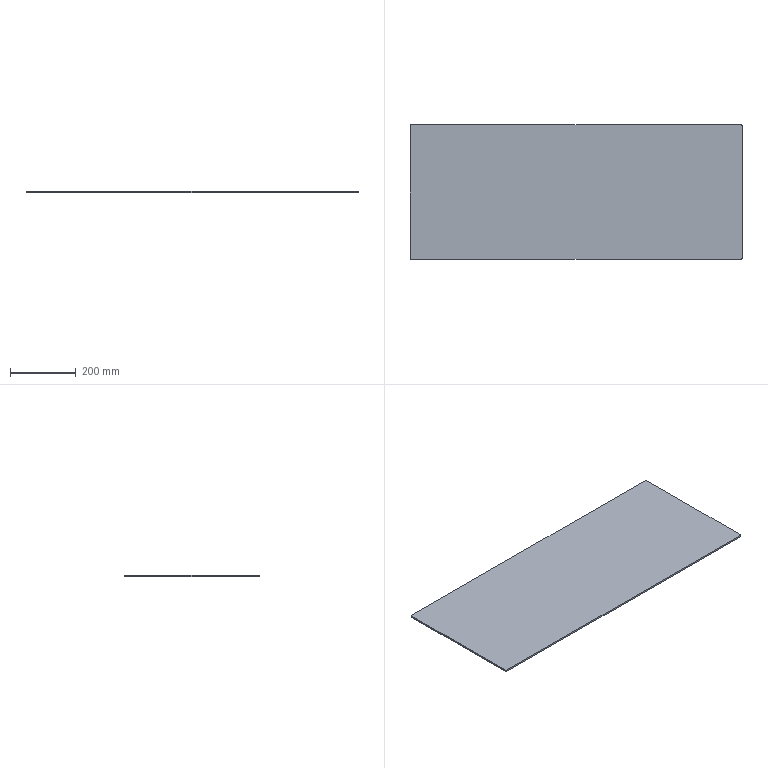Part | STEP file | rear door acrylic cover plate | 1 solid | 10 faces | box 1010 x 409 x 5 mm | volume 2065411 mm3 | plane 6 | cylinder 4 | commonest cylinder face diameters 6 x4
STEP:
#1=CARTESIAN_POINT('',(0.,0.,0.));
#2=DIRECTION('',(0.,0.,1.));
#3=DIRECTION('',(1.,0.,0.));
#4=AXIS2_PLACEMENT_3D('',#1,#2,#3);
#5=CARTESIAN_POINT('',(505.,-201.5,5.));
#6=VERTEX_POINT('',#5);
#7=CARTESIAN_POINT('',(505.,201.5,5.));
#8=VERTEX_POINT('',#7);
#9=CARTESIAN_POINT('',(505.,204.5,5.));
#10=DIRECTION('',(0.,1.,0.));
#11=VECTOR('',#10,1.);
#12=LINE('',#9,#11);
#13=CARTESIAN_POINT('',(505.,204.5,5.));
#14=DIRECTION('',(-1.,0.,0.));
#15=DIRECTION('',(0.,0.,1.));
#16=AXIS2_PLACEMENT_3D('',#13,#14,#15);
#17=PLANE('',#16);
#18=CARTESIAN_POINT('',(0.,0.));
#19=DIRECTION('',(0.,1.));
#20=VECTOR('',#19,1.);
#21=LINE('',#18,#20);
#22=(GEOMETRIC_REPRESENTATION_CONTEXT(2)PARAMETRIC_REPRESENTATION_CONTEXT()REPRESENTATION_CONTEXT('',''));
#23=DEFINITIONAL_REPRESENTATION('',(#21),#22);
#24=PCURVE('',#17,#23);
#25=CARTESIAN_POINT('',(0.,0.,5.));
#26=DIRECTION('',(0.,0.,1.));
#27=DIRECTION('',(1.,0.,0.));
#28=AXIS2_PLACEMENT_3D('',#25,#26,#27);
#29=PLANE('',#28);
#30=CARTESIAN_POINT('',(505.,204.5));
#31=DIRECTION('',(0.,1.));
#32=VECTOR('',#31,1.);
#33=LINE('',#30,#32);
#34=(GEOMETRIC_REPRESENTATION_CONTEXT(2)PARAMETRIC_REPRESENTATION_CONTEXT()REPRESENTATION_CONTEXT('',''));
#35=DEFINITIONAL_REPRESENTATION('',(#33),#34);
#36=PCURVE('',#29,#35);
#37=SURFACE_CURVE('',#12,(#24,#36),.PCURVE_S1.);
#38=EDGE_CURVE('',#6,#8,#37,.T.);
#39=ORIENTED_EDGE('',*,*,#38,.F.);
#40=CARTESIAN_POINT('',(505.,-201.5,0.));
#41=VERTEX_POINT('',#40);
#42=CARTESIAN_POINT('',(505.,-201.5,5.));
#43=DIRECTION('',(0.,0.,-1.));
#44=VECTOR('',#43,1.);
#45=LINE('',#42,#44);
#46=CARTESIAN_POINT('',(0.,-406.));
#47=DIRECTION('',(-1.,0.));
#48=VECTOR('',#47,1.);
#49=LINE('',#46,#48);
#50=(GEOMETRIC_REPRESENTATION_CONTEXT(2)PARAMETRIC_REPRESENTATION_CONTEXT()REPRESENTATION_CONTEXT('',''));
#51=DEFINITIONAL_REPRESENTATION('',(#49),#50);
#52=PCURVE('',#17,#51);
#53=CARTESIAN_POINT('',(502.,-201.5,5.));
#54=DIRECTION('',(0.,0.,-1.));
#55=DIRECTION('',(-1.,0.,0.));
#56=AXIS2_PLACEMENT_3D('',#53,#54,#55);
#57=CYLINDRICAL_SURFACE('',#56,3.);
#58=CARTESIAN_POINT('',(3.142,0.));
#59=DIRECTION('',(0.,1.));
#60=VECTOR('',#59,1.);
#61=LINE('',#58,#60);
#62=(GEOMETRIC_REPRESENTATION_CONTEXT(2)PARAMETRIC_REPRESENTATION_CONTEXT()REPRESENTATION_CONTEXT('',''));
#63=DEFINITIONAL_REPRESENTATION('',(#61),#62);
#64=PCURVE('',#57,#63);
#65=SURFACE_CURVE('',#45,(#52,#64),.PCURVE_S1.);
#66=EDGE_CURVE('',#6,#41,#65,.T.);
#67=ORIENTED_EDGE('',*,*,#66,.T.);
#68=CARTESIAN_POINT('',(505.,201.5,0.));
#69=VERTEX_POINT('',#68);
#70=CARTESIAN_POINT('',(505.,204.5,0.));
#71=DIRECTION('',(0.,1.,0.));
#72=VECTOR('',#71,1.);
#73=LINE('',#70,#72);
#74=CARTESIAN_POINT('',(-5.,0.));
#75=DIRECTION('',(0.,1.));
#76=VECTOR('',#75,1.);
#77=LINE('',#74,#76);
#78=(GEOMETRIC_REPRESENTATION_CONTEXT(2)PARAMETRIC_REPRESENTATION_CONTEXT()REPRESENTATION_CONTEXT('',''));
#79=DEFINITIONAL_REPRESENTATION('',(#77),#78);
#80=PCURVE('',#17,#79);
#81=CARTESIAN_POINT('',(0.,0.,0.));
#82=DIRECTION('',(0.,0.,1.));
#83=DIRECTION('',(1.,0.,0.));
#84=AXIS2_PLACEMENT_3D('',#81,#82,#83);
#85=PLANE('',#84);
#86=CARTESIAN_POINT('',(505.,204.5));
#87=DIRECTION('',(0.,1.));
#88=VECTOR('',#87,1.);
#89=LINE('',#86,#88);
#90=(GEOMETRIC_REPRESENTATION_CONTEXT(2)PARAMETRIC_REPRESENTATION_CONTEXT()REPRESENTATION_CONTEXT('',''));
#91=DEFINITIONAL_REPRESENTATION('',(#89),#90);
#92=PCURVE('',#85,#91);
#93=SURFACE_CURVE('',#73,(#80,#92),.PCURVE_S1.);
#94=EDGE_CURVE('',#41,#69,#93,.T.);
#95=ORIENTED_EDGE('',*,*,#94,.T.);
#96=CARTESIAN_POINT('',(505.,201.5,5.));
#97=DIRECTION('',(0.,0.,1.));
#98=VECTOR('',#97,1.);
#99=LINE('',#96,#98);
#100=CARTESIAN_POINT('',(0.,-3.));
#101=DIRECTION('',(1.,0.));
#102=VECTOR('',#101,1.);
#103=LINE('',#100,#102);
#104=(GEOMETRIC_REPRESENTATION_CONTEXT(2)PARAMETRIC_REPRESENTATION_CONTEXT()REPRESENTATION_CONTEXT('',''));
#105=DEFINITIONAL_REPRESENTATION('',(#103),#104);
#106=PCURVE('',#17,#105);
#107=CARTESIAN_POINT('',(502.,201.5,5.));
#108=DIRECTION('',(0.,0.,-1.));
#109=DIRECTION('',(-1.,0.,0.));
#110=AXIS2_PLACEMENT_3D('',#107,#108,#109);
#111=CYLINDRICAL_SURFACE('',#110,3.);
#112=CARTESIAN_POINT('',(3.142,0.));
#113=DIRECTION('',(0.,-1.));
#114=VECTOR('',#113,1.);
#115=LINE('',#112,#114);
#116=(GEOMETRIC_REPRESENTATION_CONTEXT(2)PARAMETRIC_REPRESENTATION_CONTEXT()REPRESENTATION_CONTEXT('',''));
#117=DEFINITIONAL_REPRESENTATION('',(#115),#116);
#118=PCURVE('',#111,#117);
#119=SURFACE_CURVE('',#99,(#106,#118),.PCURVE_S1.);
#120=EDGE_CURVE('',#69,#8,#119,.T.);
#121=ORIENTED_EDGE('',*,*,#120,.T.);
#122=EDGE_LOOP('',(#39,#67,#95,#121));
#123=FACE_BOUND('',#122,.T.);
#124=ADVANCED_FACE('',(#123),#17,.F.);
#125=CARTESIAN_POINT('',(502.,204.5,0.));
#126=VERTEX_POINT('',#125);
#127=CARTESIAN_POINT('',(-502.,204.5,0.));
#128=VERTEX_POINT('',#127);
#129=CARTESIAN_POINT('',(-505.,204.5,0.));
#130=DIRECTION('',(-1.,0.,0.));
#131=VECTOR('',#130,1.);
#132=LINE('',#129,#131);
#133=CARTESIAN_POINT('',(-505.,204.5,5.));
#134=DIRECTION('',(0.,-1.,0.));
#135=DIRECTION('',(0.,0.,-1.));
#136=AXIS2_PLACEMENT_3D('',#133,#134,#135);
#137=PLANE('',#136);
#138=CARTESIAN_POINT('',(5.,0.));
#139=DIRECTION('',(0.,-1.));
#140=VECTOR('',#139,1.);
#141=LINE('',#138,#140);
#142=(GEOMETRIC_REPRESENTATION_CONTEXT(2)PARAMETRIC_REPRESENTATION_CONTEXT()REPRESENTATION_CONTEXT('',''));
#143=DEFINITIONAL_REPRESENTATION('',(#141),#142);
#144=PCURVE('',#137,#143);
#145=CARTESIAN_POINT('',(-505.,204.5));
#146=DIRECTION('',(-1.,0.));
#147=VECTOR('',#146,1.);
#148=LINE('',#145,#147);
#149=(GEOMETRIC_REPRESENTATION_CONTEXT(2)PARAMETRIC_REPRESENTATION_CONTEXT()REPRESENTATION_CONTEXT('',''));
#150=DEFINITIONAL_REPRESENTATION('',(#148),#149);
#151=PCURVE('',#85,#150);
#152=SURFACE_CURVE('',#132,(#144,#151),.PCURVE_S1.);
#153=EDGE_CURVE('',#126,#128,#152,.T.);
#154=ORIENTED_EDGE('',*,*,#153,.T.);
#155=CARTESIAN_POINT('',(-502.,204.5,5.));
#156=VERTEX_POINT('',#155);
#157=CARTESIAN_POINT('',(-502.,204.5,5.));
#158=DIRECTION('',(0.,0.,1.));
#159=VECTOR('',#158,1.);
#160=LINE('',#157,#159);
#161=CARTESIAN_POINT('',(0.,3.));
#162=DIRECTION('',(-1.,0.));
#163=VECTOR('',#162,1.);
#164=LINE('',#161,#163);
#165=(GEOMETRIC_REPRESENTATION_CONTEXT(2)PARAMETRIC_REPRESENTATION_CONTEXT()REPRESENTATION_CONTEXT('',''));
#166=DEFINITIONAL_REPRESENTATION('',(#164),#165);
#167=PCURVE('',#137,#166);
#168=CARTESIAN_POINT('',(-502.,201.5,5.));
#169=DIRECTION('',(0.,0.,-1.));
#170=DIRECTION('',(-1.,0.,0.));
#171=AXIS2_PLACEMENT_3D('',#168,#169,#170);
#172=CYLINDRICAL_SURFACE('',#171,3.);
#173=CARTESIAN_POINT('',(1.571,0.));
#174=DIRECTION('',(0.,-1.));
#175=VECTOR('',#174,1.);
#176=LINE('',#173,#175);
#177=(GEOMETRIC_REPRESENTATION_CONTEXT(2)PARAMETRIC_REPRESENTATION_CONTEXT()REPRESENTATION_CONTEXT('',''));
#178=DEFINITIONAL_REPRESENTATION('',(#176),#177);
#179=PCURVE('',#172,#178);
#180=SURFACE_CURVE('',#160,(#167,#179),.PCURVE_S1.);
#181=EDGE_CURVE('',#128,#156,#180,.T.);
#182=ORIENTED_EDGE('',*,*,#181,.T.);
#183=CARTESIAN_POINT('',(502.,204.5,5.));
#184=VERTEX_POINT('',#183);
#185=CARTESIAN_POINT('',(-505.,204.5,5.));
#186=DIRECTION('',(-1.,0.,0.));
#187=VECTOR('',#186,1.);
#188=LINE('',#185,#187);
#189=CARTESIAN_POINT('',(0.,0.));
#190=DIRECTION('',(0.,-1.));
#191=VECTOR('',#190,1.);
#192=LINE('',#189,#191);
#193=(GEOMETRIC_REPRESENTATION_CONTEXT(2)PARAMETRIC_REPRESENTATION_CONTEXT()REPRESENTATION_CONTEXT('',''));
#194=DEFINITIONAL_REPRESENTATION('',(#192),#193);
#195=PCURVE('',#137,#194);
#196=CARTESIAN_POINT('',(-505.,204.5));
#197=DIRECTION('',(-1.,0.));
#198=VECTOR('',#197,1.);
#199=LINE('',#196,#198);
#200=(GEOMETRIC_REPRESENTATION_CONTEXT(2)PARAMETRIC_REPRESENTATION_CONTEXT()REPRESENTATION_CONTEXT('',''));
#201=DEFINITIONAL_REPRESENTATION('',(#199),#200);
#202=PCURVE('',#29,#201);
#203=SURFACE_CURVE('',#188,(#195,#202),.PCURVE_S1.);
#204=EDGE_CURVE('',#184,#156,#203,.T.);
#205=ORIENTED_EDGE('',*,*,#204,.F.);
#206=CARTESIAN_POINT('',(502.,204.5,5.));
#207=DIRECTION('',(0.,0.,-1.));
#208=VECTOR('',#207,1.);
#209=LINE('',#206,#208);
#210=CARTESIAN_POINT('',(0.,1007.));
#211=DIRECTION('',(1.,0.));
#212=VECTOR('',#211,1.);
#213=LINE('',#210,#212);
#214=(GEOMETRIC_REPRESENTATION_CONTEXT(2)PARAMETRIC_REPRESENTATION_CONTEXT()REPRESENTATION_CONTEXT('',''));
#215=DEFINITIONAL_REPRESENTATION('',(#213),#214);
#216=PCURVE('',#137,#215);
#217=CARTESIAN_POINT('',(1.571,0.));
#218=DIRECTION('',(0.,1.));
#219=VECTOR('',#218,1.);
#220=LINE('',#217,#219);
#221=(GEOMETRIC_REPRESENTATION_CONTEXT(2)PARAMETRIC_REPRESENTATION_CONTEXT()REPRESENTATION_CONTEXT('',''));
#222=DEFINITIONAL_REPRESENTATION('',(#220),#221);
#223=PCURVE('',#111,#222);
#224=SURFACE_CURVE('',#209,(#216,#223),.PCURVE_S1.);
#225=EDGE_CURVE('',#184,#126,#224,.T.);
#226=ORIENTED_EDGE('',*,*,#225,.T.);
#227=EDGE_LOOP('',(#154,#182,#205,#226));
#228=FACE_BOUND('',#227,.T.);
#229=ADVANCED_FACE('',(#228),#137,.F.);
#230=CARTESIAN_POINT('',(-505.,201.5,5.));
#231=VERTEX_POINT('',#230);
#232=CARTESIAN_POINT('',(-505.,-201.5,5.));
#233=VERTEX_POINT('',#232);
#234=CARTESIAN_POINT('',(-505.,204.5,5.));
#235=DIRECTION('',(0.,-1.,0.));
#236=VECTOR('',#235,1.);
#237=LINE('',#234,#236);
#238=CARTESIAN_POINT('',(-505.,204.5,5.));
#239=DIRECTION('',(1.,0.,0.));
#240=DIRECTION('',(0.,1.,0.));
#241=AXIS2_PLACEMENT_3D('',#238,#239,#240);
#242=PLANE('',#241);
#243=CARTESIAN_POINT('',(0.,0.));
#244=DIRECTION('',(-1.,0.));
#245=VECTOR('',#244,1.);
#246=LINE('',#243,#245);
#247=(GEOMETRIC_REPRESENTATION_CONTEXT(2)PARAMETRIC_REPRESENTATION_CONTEXT()REPRESENTATION_CONTEXT('',''));
#248=DEFINITIONAL_REPRESENTATION('',(#246),#247);
#249=PCURVE('',#242,#248);
#250=CARTESIAN_POINT('',(-505.,204.5));
#251=DIRECTION('',(0.,-1.));
#252=VECTOR('',#251,1.);
#253=LINE('',#250,#252);
#254=(GEOMETRIC_REPRESENTATION_CONTEXT(2)PARAMETRIC_REPRESENTATION_CONTEXT()REPRESENTATION_CONTEXT('',''));
#255=DEFINITIONAL_REPRESENTATION('',(#253),#254);
#256=PCURVE('',#29,#255);
#257=SURFACE_CURVE('',#237,(#249,#256),.PCURVE_S1.);
#258=EDGE_CURVE('',#231,#233,#257,.T.);
#259=ORIENTED_EDGE('',*,*,#258,.F.);
#260=CARTESIAN_POINT('',(-505.,201.5,0.));
#261=VERTEX_POINT('',#260);
#262=CARTESIAN_POINT('',(-505.,201.5,5.));
#263=DIRECTION('',(0.,0.,-1.));
#264=VECTOR('',#263,1.);
#265=LINE('',#262,#264);
#266=CARTESIAN_POINT('',(-3.,0.));
#267=DIRECTION('',(0.,-1.));
#268=VECTOR('',#267,1.);
#269=LINE('',#266,#268);
#270=(GEOMETRIC_REPRESENTATION_CONTEXT(2)PARAMETRIC_REPRESENTATION_CONTEXT()REPRESENTATION_CONTEXT('',''));
#271=DEFINITIONAL_REPRESENTATION('',(#269),#270);
#272=PCURVE('',#242,#271);
#273=CARTESIAN_POINT('',(0.,0.));
#274=DIRECTION('',(0.,1.));
#275=VECTOR('',#274,1.);
#276=LINE('',#273,#275);
#277=(GEOMETRIC_REPRESENTATION_CONTEXT(2)PARAMETRIC_REPRESENTATION_CONTEXT()REPRESENTATION_CONTEXT('',''));
#278=DEFINITIONAL_REPRESENTATION('',(#276),#277);
#279=PCURVE('',#172,#278);
#280=SURFACE_CURVE('',#265,(#272,#279),.PCURVE_S1.);
#281=EDGE_CURVE('',#231,#261,#280,.T.);
#282=ORIENTED_EDGE('',*,*,#281,.T.);
#283=CARTESIAN_POINT('',(-505.,-201.5,0.));
#284=VERTEX_POINT('',#283);
#285=CARTESIAN_POINT('',(-505.,204.5,0.));
#286=DIRECTION('',(0.,-1.,0.));
#287=VECTOR('',#286,1.);
#288=LINE('',#285,#287);
#289=CARTESIAN_POINT('',(0.,-5.));
#290=DIRECTION('',(-1.,0.));
#291=VECTOR('',#290,1.);
#292=LINE('',#289,#291);
#293=(GEOMETRIC_REPRESENTATION_CONTEXT(2)PARAMETRIC_REPRESENTATION_CONTEXT()REPRESENTATION_CONTEXT('',''));
#294=DEFINITIONAL_REPRESENTATION('',(#292),#293);
#295=PCURVE('',#242,#294);
#296=CARTESIAN_POINT('',(-505.,204.5));
#297=DIRECTION('',(0.,-1.));
#298=VECTOR('',#297,1.);
#299=LINE('',#296,#298);
#300=(GEOMETRIC_REPRESENTATION_CONTEXT(2)PARAMETRIC_REPRESENTATION_CONTEXT()REPRESENTATION_CONTEXT('',''));
#301=DEFINITIONAL_REPRESENTATION('',(#299),#300);
#302=PCURVE('',#85,#301);
#303=SURFACE_CURVE('',#288,(#295,#302),.PCURVE_S1.);
#304=EDGE_CURVE('',#261,#284,#303,.T.);
#305=ORIENTED_EDGE('',*,*,#304,.T.);
#306=CARTESIAN_POINT('',(-505.,-201.5,5.));
#307=DIRECTION('',(0.,0.,1.));
#308=VECTOR('',#307,1.);
#309=LINE('',#306,#308);
#310=CARTESIAN_POINT('',(-406.,0.));
#311=DIRECTION('',(0.,1.));
#312=VECTOR('',#311,1.);
#313=LINE('',#310,#312);
#314=(GEOMETRIC_REPRESENTATION_CONTEXT(2)PARAMETRIC_REPRESENTATION_CONTEXT()REPRESENTATION_CONTEXT('',''));
#315=DEFINITIONAL_REPRESENTATION('',(#313),#314);
#316=PCURVE('',#242,#315);
#317=CARTESIAN_POINT('',(-502.,-201.5,5.));
#318=DIRECTION('',(0.,0.,-1.));
#319=DIRECTION('',(-1.,0.,0.));
#320=AXIS2_PLACEMENT_3D('',#317,#318,#319);
#321=CYLINDRICAL_SURFACE('',#320,3.);
#322=CARTESIAN_POINT('',(6.283,0.));
#323=DIRECTION('',(0.,-1.));
#324=VECTOR('',#323,1.);
#325=LINE('',#322,#324);
#326=(GEOMETRIC_REPRESENTATION_CONTEXT(2)PARAMETRIC_REPRESENTATION_CONTEXT()REPRESENTATION_CONTEXT('',''));
#327=DEFINITIONAL_REPRESENTATION('',(#325),#326);
#328=PCURVE('',#321,#327);
#329=SURFACE_CURVE('',#309,(#316,#328),.PCURVE_S1.);
#330=EDGE_CURVE('',#284,#233,#329,.T.);
#331=ORIENTED_EDGE('',*,*,#330,.T.);
#332=EDGE_LOOP('',(#259,#282,#305,#331));
#333=FACE_BOUND('',#332,.T.);
#334=ADVANCED_FACE('',(#333),#242,.F.);
#335=CARTESIAN_POINT('',(-502.,-204.5,5.));
#336=VERTEX_POINT('',#335);
#337=CARTESIAN_POINT('',(502.,-204.5,5.));
#338=VERTEX_POINT('',#337);
#339=CARTESIAN_POINT('',(-505.,-204.5,5.));
#340=DIRECTION('',(1.,0.,0.));
#341=VECTOR('',#340,1.);
#342=LINE('',#339,#341);
#343=CARTESIAN_POINT('',(-505.,-204.5,5.));
#344=DIRECTION('',(0.,1.,0.));
#345=DIRECTION('',(0.,0.,1.));
#346=AXIS2_PLACEMENT_3D('',#343,#344,#345);
#347=PLANE('',#346);
#348=CARTESIAN_POINT('',(0.,0.));
#349=DIRECTION('',(0.,1.));
#350=VECTOR('',#349,1.);
#351=LINE('',#348,#350);
#352=(GEOMETRIC_REPRESENTATION_CONTEXT(2)PARAMETRIC_REPRESENTATION_CONTEXT()REPRESENTATION_CONTEXT('',''));
#353=DEFINITIONAL_REPRESENTATION('',(#351),#352);
#354=PCURVE('',#347,#353);
#355=CARTESIAN_POINT('',(-505.,-204.5));
#356=DIRECTION('',(1.,0.));
#357=VECTOR('',#356,1.);
#358=LINE('',#355,#357);
#359=(GEOMETRIC_REPRESENTATION_CONTEXT(2)PARAMETRIC_REPRESENTATION_CONTEXT()REPRESENTATION_CONTEXT('',''));
#360=DEFINITIONAL_REPRESENTATION('',(#358),#359);
#361=PCURVE('',#29,#360);
#362=SURFACE_CURVE('',#342,(#354,#361),.PCURVE_S1.);
#363=EDGE_CURVE('',#336,#338,#362,.T.);
#364=ORIENTED_EDGE('',*,*,#363,.F.);
#365=CARTESIAN_POINT('',(-502.,-204.5,0.));
#366=VERTEX_POINT('',#365);
#367=CARTESIAN_POINT('',(-502.,-204.5,5.));
#368=DIRECTION('',(0.,0.,-1.));
#369=VECTOR('',#368,1.);
#370=LINE('',#367,#369);
#371=CARTESIAN_POINT('',(0.,3.));
#372=DIRECTION('',(-1.,0.));
#373=VECTOR('',#372,1.);
#374=LINE('',#371,#373);
#375=(GEOMETRIC_REPRESENTATION_CONTEXT(2)PARAMETRIC_REPRESENTATION_CONTEXT()REPRESENTATION_CONTEXT('',''));
#376=DEFINITIONAL_REPRESENTATION('',(#374),#375);
#377=PCURVE('',#347,#376);
#378=CARTESIAN_POINT('',(4.712,0.));
#379=DIRECTION('',(0.,1.));
#380=VECTOR('',#379,1.);
#381=LINE('',#378,#380);
#382=(GEOMETRIC_REPRESENTATION_CONTEXT(2)PARAMETRIC_REPRESENTATION_CONTEXT()REPRESENTATION_CONTEXT('',''));
#383=DEFINITIONAL_REPRESENTATION('',(#381),#382);
#384=PCURVE('',#321,#383);
#385=SURFACE_CURVE('',#370,(#377,#384),.PCURVE_S1.);
#386=EDGE_CURVE('',#336,#366,#385,.T.);
#387=ORIENTED_EDGE('',*,*,#386,.T.);
#388=CARTESIAN_POINT('',(502.,-204.5,0.));
#389=VERTEX_POINT('',#388);
#390=CARTESIAN_POINT('',(-505.,-204.5,0.));
#391=DIRECTION('',(1.,0.,0.));
#392=VECTOR('',#391,1.);
#393=LINE('',#390,#392);
#394=CARTESIAN_POINT('',(-5.,0.));
#395=DIRECTION('',(0.,1.));
#396=VECTOR('',#395,1.);
#397=LINE('',#394,#396);
#398=(GEOMETRIC_REPRESENTATION_CONTEXT(2)PARAMETRIC_REPRESENTATION_CONTEXT()REPRESENTATION_CONTEXT('',''));
#399=DEFINITIONAL_REPRESENTATION('',(#397),#398);
#400=PCURVE('',#347,#399);
#401=CARTESIAN_POINT('',(-505.,-204.5));
#402=DIRECTION('',(1.,0.));
#403=VECTOR('',#402,1.);
#404=LINE('',#401,#403);
#405=(GEOMETRIC_REPRESENTATION_CONTEXT(2)PARAMETRIC_REPRESENTATION_CONTEXT()REPRESENTATION_CONTEXT('',''));
#406=DEFINITIONAL_REPRESENTATION('',(#404),#405);
#407=PCURVE('',#85,#406);
#408=SURFACE_CURVE('',#393,(#400,#407),.PCURVE_S1.);
#409=EDGE_CURVE('',#366,#389,#408,.T.);
#410=ORIENTED_EDGE('',*,*,#409,.T.);
#411=CARTESIAN_POINT('',(502.,-204.5,5.));
#412=DIRECTION('',(0.,0.,1.));
#413=VECTOR('',#412,1.);
#414=LINE('',#411,#413);
#415=CARTESIAN_POINT('',(0.,1007.));
#416=DIRECTION('',(1.,0.));
#417=VECTOR('',#416,1.);
#418=LINE('',#415,#417);
#419=(GEOMETRIC_REPRESENTATION_CONTEXT(2)PARAMETRIC_REPRESENTATION_CONTEXT()REPRESENTATION_CONTEXT('',''));
#420=DEFINITIONAL_REPRESENTATION('',(#418),#419);
#421=PCURVE('',#347,#420);
#422=CARTESIAN_POINT('',(4.712,0.));
#423=DIRECTION('',(0.,-1.));
#424=VECTOR('',#423,1.);
#425=LINE('',#422,#424);
#426=(GEOMETRIC_REPRESENTATION_CONTEXT(2)PARAMETRIC_REPRESENTATION_CONTEXT()REPRESENTATION_CONTEXT('',''));
#427=DEFINITIONAL_REPRESENTATION('',(#425),#426);
#428=PCURVE('',#57,#427);
#429=SURFACE_CURVE('',#414,(#421,#428),.PCURVE_S1.);
#430=EDGE_CURVE('',#389,#338,#429,.T.);
#431=ORIENTED_EDGE('',*,*,#430,.T.);
#432=EDGE_LOOP('',(#364,#387,#410,#431));
#433=FACE_BOUND('',#432,.T.);
#434=ADVANCED_FACE('',(#433),#347,.F.);
#435=ORIENTED_EDGE('',*,*,#204,.T.);
#436=CARTESIAN_POINT('',(-502.,201.5,5.));
#437=DIRECTION('',(0.,0.,1.));
#438=DIRECTION('',(1.,0.,0.));
#439=AXIS2_PLACEMENT_3D('',#436,#437,#438);
#440=CIRCLE('',#439,3.);
#441=CARTESIAN_POINT('',(-502.,201.5));
#442=DIRECTION('',(1.,0.));
#443=AXIS2_PLACEMENT_2D('',#441,#442);
#444=CIRCLE('',#443,3.);
#445=(GEOMETRIC_REPRESENTATION_CONTEXT(2)PARAMETRIC_REPRESENTATION_CONTEXT()REPRESENTATION_CONTEXT('',''));
#446=DEFINITIONAL_REPRESENTATION('',(#444),#445);
#447=PCURVE('',#29,#446);
#448=CARTESIAN_POINT('',(3.142,0.));
#449=DIRECTION('',(-1.,0.));
#450=VECTOR('',#449,1.);
#451=LINE('',#448,#450);
#452=(GEOMETRIC_REPRESENTATION_CONTEXT(2)PARAMETRIC_REPRESENTATION_CONTEXT()REPRESENTATION_CONTEXT('',''));
#453=DEFINITIONAL_REPRESENTATION('',(#451),#452);
#454=PCURVE('',#172,#453);
#455=SURFACE_CURVE('',#440,(#447,#454),.PCURVE_S1.);
#456=EDGE_CURVE('',#156,#231,#455,.T.);
#457=ORIENTED_EDGE('',*,*,#456,.T.);
#458=ORIENTED_EDGE('',*,*,#258,.T.);
#459=CARTESIAN_POINT('',(-502.,-201.5,5.));
#460=DIRECTION('',(0.,0.,1.));
#461=DIRECTION('',(1.,0.,0.));
#462=AXIS2_PLACEMENT_3D('',#459,#460,#461);
#463=CIRCLE('',#462,3.);
#464=CARTESIAN_POINT('',(-502.,-201.5));
#465=DIRECTION('',(1.,0.));
#466=AXIS2_PLACEMENT_2D('',#464,#465);
#467=CIRCLE('',#466,3.);
#468=(GEOMETRIC_REPRESENTATION_CONTEXT(2)PARAMETRIC_REPRESENTATION_CONTEXT()REPRESENTATION_CONTEXT('',''));
#469=DEFINITIONAL_REPRESENTATION('',(#467),#468);
#470=PCURVE('',#29,#469);
#471=CARTESIAN_POINT('',(9.425,0.));
#472=DIRECTION('',(-1.,0.));
#473=VECTOR('',#472,1.);
#474=LINE('',#471,#473);
#475=(GEOMETRIC_REPRESENTATION_CONTEXT(2)PARAMETRIC_REPRESENTATION_CONTEXT()REPRESENTATION_CONTEXT('',''));
#476=DEFINITIONAL_REPRESENTATION('',(#474),#475);
#477=PCURVE('',#321,#476);
#478=SURFACE_CURVE('',#463,(#470,#477),.PCURVE_S1.);
#479=EDGE_CURVE('',#233,#336,#478,.T.);
#480=ORIENTED_EDGE('',*,*,#479,.T.);
#481=ORIENTED_EDGE('',*,*,#363,.T.);
#482=CARTESIAN_POINT('',(502.,-201.5,5.));
#483=DIRECTION('',(0.,0.,1.));
#484=DIRECTION('',(1.,0.,0.));
#485=AXIS2_PLACEMENT_3D('',#482,#483,#484);
#486=CIRCLE('',#485,3.);
#487=CARTESIAN_POINT('',(502.,-201.5));
#488=DIRECTION('',(1.,0.));
#489=AXIS2_PLACEMENT_2D('',#487,#488);
#490=CIRCLE('',#489,3.);
#491=(GEOMETRIC_REPRESENTATION_CONTEXT(2)PARAMETRIC_REPRESENTATION_CONTEXT()REPRESENTATION_CONTEXT('',''));
#492=DEFINITIONAL_REPRESENTATION('',(#490),#491);
#493=PCURVE('',#29,#492);
#494=CARTESIAN_POINT('',(9.425,0.));
#495=DIRECTION('',(-1.,0.));
#496=VECTOR('',#495,1.);
#497=LINE('',#494,#496);
#498=(GEOMETRIC_REPRESENTATION_CONTEXT(2)PARAMETRIC_REPRESENTATION_CONTEXT()REPRESENTATION_CONTEXT('',''));
#499=DEFINITIONAL_REPRESENTATION('',(#497),#498);
#500=PCURVE('',#57,#499);
#501=SURFACE_CURVE('',#486,(#493,#500),.PCURVE_S1.);
#502=EDGE_CURVE('',#338,#6,#501,.T.);
#503=ORIENTED_EDGE('',*,*,#502,.T.);
#504=ORIENTED_EDGE('',*,*,#38,.T.);
#505=CARTESIAN_POINT('',(502.,201.5,5.));
#506=DIRECTION('',(0.,0.,1.));
#507=DIRECTION('',(1.,0.,0.));
#508=AXIS2_PLACEMENT_3D('',#505,#506,#507);
#509=CIRCLE('',#508,3.);
#510=CARTESIAN_POINT('',(502.,201.5));
#511=DIRECTION('',(1.,0.));
#512=AXIS2_PLACEMENT_2D('',#510,#511);
#513=CIRCLE('',#512,3.);
#514=(GEOMETRIC_REPRESENTATION_CONTEXT(2)PARAMETRIC_REPRESENTATION_CONTEXT()REPRESENTATION_CONTEXT('',''));
#515=DEFINITIONAL_REPRESENTATION('',(#513),#514);
#516=PCURVE('',#29,#515);
#517=CARTESIAN_POINT('',(3.142,0.));
#518=DIRECTION('',(-1.,0.));
#519=VECTOR('',#518,1.);
#520=LINE('',#517,#519);
#521=(GEOMETRIC_REPRESENTATION_CONTEXT(2)PARAMETRIC_REPRESENTATION_CONTEXT()REPRESENTATION_CONTEXT('',''));
#522=DEFINITIONAL_REPRESENTATION('',(#520),#521);
#523=PCURVE('',#111,#522);
#524=SURFACE_CURVE('',#509,(#516,#523),.PCURVE_S1.);
#525=EDGE_CURVE('',#8,#184,#524,.T.);
#526=ORIENTED_EDGE('',*,*,#525,.T.);
#527=EDGE_LOOP('',(#435,#457,#458,#480,#481,#503,#504,#526));
#528=FACE_BOUND('',#527,.T.);
#529=ADVANCED_FACE('',(#528),#29,.T.);
#530=ORIENTED_EDGE('',*,*,#304,.F.);
#531=CARTESIAN_POINT('',(-502.,201.5,0.));
#532=DIRECTION('',(0.,0.,-1.));
#533=DIRECTION('',(1.,0.,0.));
#534=AXIS2_PLACEMENT_3D('',#531,#532,#533);
#535=CIRCLE('',#534,3.);
#536=CARTESIAN_POINT('',(-499.,201.5));
#537=CARTESIAN_POINT('',(-499.,196.304));
#538=CARTESIAN_POINT('',(-503.5,198.902));
#539=CARTESIAN_POINT('',(-508.,201.5));
#540=CARTESIAN_POINT('',(-503.5,204.098));
#541=CARTESIAN_POINT('',(-499.,206.696));
#542=CARTESIAN_POINT('',(-499.,201.5));
#543=(BOUNDED_CURVE()B_SPLINE_CURVE(2,(#536,#537,#538,#539,#540,#541,#542),.UNSPECIFIED.,.T.,.F.)B_SPLINE_CURVE_WITH_KNOTS((1,2,2,2,2,1),(-2.094,0.,2.094,4.189,6.283,8.378),.UNSPECIFIED.)CURVE()GEOMETRIC_REPRESENTATION_ITEM()RATIONAL_B_SPLINE_CURVE((1.,0.5,1.,0.5,1.,0.5,1.))REPRESENTATION_ITEM(''));
#544=(GEOMETRIC_REPRESENTATION_CONTEXT(2)PARAMETRIC_REPRESENTATION_CONTEXT()REPRESENTATION_CONTEXT('',''));
#545=DEFINITIONAL_REPRESENTATION('',(#543),#544);
#546=PCURVE('',#85,#545);
#547=CARTESIAN_POINT('',(-3.142,5.));
#548=DIRECTION('',(1.,0.));
#549=VECTOR('',#548,1.);
#550=LINE('',#547,#549);
#551=(GEOMETRIC_REPRESENTATION_CONTEXT(2)PARAMETRIC_REPRESENTATION_CONTEXT()REPRESENTATION_CONTEXT('',''));
#552=DEFINITIONAL_REPRESENTATION('',(#550),#551);
#553=PCURVE('',#172,#552);
#554=SURFACE_CURVE('',#535,(#546,#553),.PCURVE_S1.);
#555=EDGE_CURVE('',#261,#128,#554,.T.);
#556=ORIENTED_EDGE('',*,*,#555,.T.);
#557=ORIENTED_EDGE('',*,*,#153,.F.);
#558=CARTESIAN_POINT('',(502.,201.5,0.));
#559=DIRECTION('',(0.,0.,-1.));
#560=DIRECTION('',(1.,0.,0.));
#561=AXIS2_PLACEMENT_3D('',#558,#559,#560);
#562=CIRCLE('',#561,3.);
#563=CARTESIAN_POINT('',(505.,201.5));
#564=CARTESIAN_POINT('',(505.,196.304));
#565=CARTESIAN_POINT('',(500.5,198.902));
#566=CARTESIAN_POINT('',(496.,201.5));
#567=CARTESIAN_POINT('',(500.5,204.098));
#568=CARTESIAN_POINT('',(505.,206.696));
#569=CARTESIAN_POINT('',(505.,201.5));
#570=(BOUNDED_CURVE()B_SPLINE_CURVE(2,(#563,#564,#565,#566,#567,#568,#569),.UNSPECIFIED.,.T.,.F.)B_SPLINE_CURVE_WITH_KNOTS((1,2,2,2,2,1),(-2.094,0.,2.094,4.189,6.283,8.378),.UNSPECIFIED.)CURVE()GEOMETRIC_REPRESENTATION_ITEM()RATIONAL_B_SPLINE_CURVE((1.,0.5,1.,0.5,1.,0.5,1.))REPRESENTATION_ITEM(''));
#571=(GEOMETRIC_REPRESENTATION_CONTEXT(2)PARAMETRIC_REPRESENTATION_CONTEXT()REPRESENTATION_CONTEXT('',''));
#572=DEFINITIONAL_REPRESENTATION('',(#570),#571);
#573=PCURVE('',#85,#572);
#574=CARTESIAN_POINT('',(-3.142,5.));
#575=DIRECTION('',(1.,0.));
#576=VECTOR('',#575,1.);
#577=LINE('',#574,#576);
#578=(GEOMETRIC_REPRESENTATION_CONTEXT(2)PARAMETRIC_REPRESENTATION_CONTEXT()REPRESENTATION_CONTEXT('',''));
#579=DEFINITIONAL_REPRESENTATION('',(#577),#578);
#580=PCURVE('',#111,#579);
#581=SURFACE_CURVE('',#562,(#573,#580),.PCURVE_S1.);
#582=EDGE_CURVE('',#126,#69,#581,.T.);
#583=ORIENTED_EDGE('',*,*,#582,.T.);
#584=ORIENTED_EDGE('',*,*,#94,.F.);
#585=CARTESIAN_POINT('',(502.,-201.5,0.));
#586=DIRECTION('',(0.,0.,-1.));
#587=DIRECTION('',(1.,0.,0.));
#588=AXIS2_PLACEMENT_3D('',#585,#586,#587);
#589=CIRCLE('',#588,3.);
#590=CARTESIAN_POINT('',(505.,-201.5));
#591=CARTESIAN_POINT('',(505.,-206.696));
#592=CARTESIAN_POINT('',(500.5,-204.098));
#593=CARTESIAN_POINT('',(496.,-201.5));
#594=CARTESIAN_POINT('',(500.5,-198.902));
#595=CARTESIAN_POINT('',(505.,-196.304));
#596=CARTESIAN_POINT('',(505.,-201.5));
#597=(BOUNDED_CURVE()B_SPLINE_CURVE(2,(#590,#591,#592,#593,#594,#595,#596),.UNSPECIFIED.,.T.,.F.)B_SPLINE_CURVE_WITH_KNOTS((1,2,2,2,2,1),(-2.094,0.,2.094,4.189,6.283,8.378),.UNSPECIFIED.)CURVE()GEOMETRIC_REPRESENTATION_ITEM()RATIONAL_B_SPLINE_CURVE((1.,0.5,1.,0.5,1.,0.5,1.))REPRESENTATION_ITEM(''));
#598=(GEOMETRIC_REPRESENTATION_CONTEXT(2)PARAMETRIC_REPRESENTATION_CONTEXT()REPRESENTATION_CONTEXT('',''));
#599=DEFINITIONAL_REPRESENTATION('',(#597),#598);
#600=PCURVE('',#85,#599);
#601=CARTESIAN_POINT('',(3.142,5.));
#602=DIRECTION('',(1.,0.));
#603=VECTOR('',#602,1.);
#604=LINE('',#601,#603);
#605=(GEOMETRIC_REPRESENTATION_CONTEXT(2)PARAMETRIC_REPRESENTATION_CONTEXT()REPRESENTATION_CONTEXT('',''));
#606=DEFINITIONAL_REPRESENTATION('',(#604),#605);
#607=PCURVE('',#57,#606);
#608=SURFACE_CURVE('',#589,(#600,#607),.PCURVE_S1.);
#609=EDGE_CURVE('',#41,#389,#608,.T.);
#610=ORIENTED_EDGE('',*,*,#609,.T.);
#611=ORIENTED_EDGE('',*,*,#409,.F.);
#612=CARTESIAN_POINT('',(-502.,-201.5,0.));
#613=DIRECTION('',(0.,0.,-1.));
#614=DIRECTION('',(1.,0.,0.));
#615=AXIS2_PLACEMENT_3D('',#612,#613,#614);
#616=CIRCLE('',#615,3.);
#617=CARTESIAN_POINT('',(-499.,-201.5));
#618=CARTESIAN_POINT('',(-499.,-206.696));
#619=CARTESIAN_POINT('',(-503.5,-204.098));
#620=CARTESIAN_POINT('',(-508.,-201.5));
#621=CARTESIAN_POINT('',(-503.5,-198.902));
#622=CARTESIAN_POINT('',(-499.,-196.304));
#623=CARTESIAN_POINT('',(-499.,-201.5));
#624=(BOUNDED_CURVE()B_SPLINE_CURVE(2,(#617,#618,#619,#620,#621,#622,#623),.UNSPECIFIED.,.T.,.F.)B_SPLINE_CURVE_WITH_KNOTS((1,2,2,2,2,1),(-2.094,0.,2.094,4.189,6.283,8.378),.UNSPECIFIED.)CURVE()GEOMETRIC_REPRESENTATION_ITEM()RATIONAL_B_SPLINE_CURVE((1.,0.5,1.,0.5,1.,0.5,1.))REPRESENTATION_ITEM(''));
#625=(GEOMETRIC_REPRESENTATION_CONTEXT(2)PARAMETRIC_REPRESENTATION_CONTEXT()REPRESENTATION_CONTEXT('',''));
#626=DEFINITIONAL_REPRESENTATION('',(#624),#625);
#627=PCURVE('',#85,#626);
#628=CARTESIAN_POINT('',(3.142,5.));
#629=DIRECTION('',(1.,0.));
#630=VECTOR('',#629,1.);
#631=LINE('',#628,#630);
#632=(GEOMETRIC_REPRESENTATION_CONTEXT(2)PARAMETRIC_REPRESENTATION_CONTEXT()REPRESENTATION_CONTEXT('',''));
#633=DEFINITIONAL_REPRESENTATION('',(#631),#632);
#634=PCURVE('',#321,#633);
#635=SURFACE_CURVE('',#616,(#627,#634),.PCURVE_S1.);
#636=EDGE_CURVE('',#366,#284,#635,.T.);
#637=ORIENTED_EDGE('',*,*,#636,.T.);
#638=EDGE_LOOP('',(#530,#556,#557,#583,#584,#610,#611,#637));
#639=FACE_BOUND('',#638,.T.);
#640=ADVANCED_FACE('',(#639),#85,.F.);
#641=ORIENTED_EDGE('',*,*,#456,.F.);
#642=ORIENTED_EDGE('',*,*,#181,.F.);
#643=ORIENTED_EDGE('',*,*,#555,.F.);
#644=ORIENTED_EDGE('',*,*,#281,.F.);
#645=EDGE_LOOP('',(#641,#642,#643,#644));
#646=FACE_BOUND('',#645,.T.);
#647=ADVANCED_FACE('',(#646),#172,.T.);
#648=ORIENTED_EDGE('',*,*,#479,.F.);
#649=ORIENTED_EDGE('',*,*,#330,.F.);
#650=ORIENTED_EDGE('',*,*,#636,.F.);
#651=ORIENTED_EDGE('',*,*,#386,.F.);
#652=EDGE_LOOP('',(#648,#649,#650,#651));
#653=FACE_BOUND('',#652,.T.);
#654=ADVANCED_FACE('',(#653),#321,.T.);
#655=ORIENTED_EDGE('',*,*,#502,.F.);
#656=ORIENTED_EDGE('',*,*,#430,.F.);
#657=ORIENTED_EDGE('',*,*,#609,.F.);
#658=ORIENTED_EDGE('',*,*,#66,.F.);
#659=EDGE_LOOP('',(#655,#656,#657,#658));
#660=FACE_BOUND('',#659,.T.);
#661=ADVANCED_FACE('',(#660),#57,.T.);
#662=ORIENTED_EDGE('',*,*,#525,.F.);
#663=ORIENTED_EDGE('',*,*,#120,.F.);
#664=ORIENTED_EDGE('',*,*,#582,.F.);
#665=ORIENTED_EDGE('',*,*,#225,.F.);
#666=EDGE_LOOP('',(#662,#663,#664,#665));
#667=FACE_BOUND('',#666,.T.);
#668=ADVANCED_FACE('',(#667),#111,.T.);
#669=CLOSED_SHELL('',(#124,#229,#334,#434,#529,#640,#647,#654,#661,#668));
#670=MANIFOLD_SOLID_BREP('',#669);
#671=(LENGTH_UNIT()NAMED_UNIT(*)SI_UNIT(.MILLI.,.METRE.));
#672=UNCERTAINTY_MEASURE_WITH_UNIT(LENGTH_MEASURE(0.0000001),#671,'','');
#673=(NAMED_UNIT(*)PLANE_ANGLE_UNIT()SI_UNIT($,.RADIAN.));
#674=(NAMED_UNIT(*)SI_UNIT($,.STERADIAN.)SOLID_ANGLE_UNIT());
#675=(GEOMETRIC_REPRESENTATION_CONTEXT(3)GLOBAL_UNCERTAINTY_ASSIGNED_CONTEXT((#672))GLOBAL_UNIT_ASSIGNED_CONTEXT((#671,#673,#674))REPRESENTATION_CONTEXT('',''));
#676=ADVANCED_BREP_SHAPE_REPRESENTATION('',(#4,#670),#675);